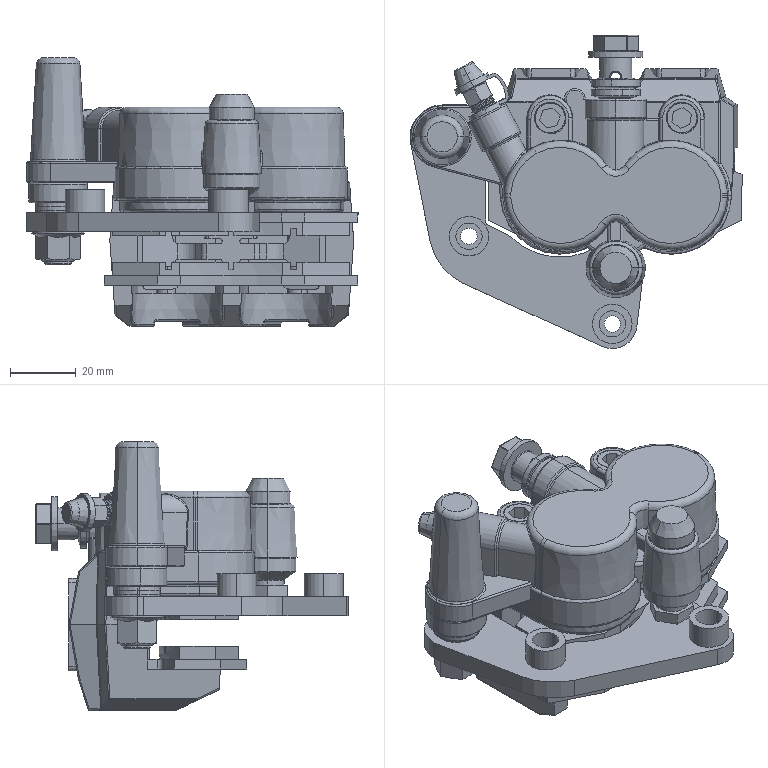Part | SolidWorks | 20 solids | 1156 faces | box 100.773 x 95.04 x 81.512 mm | volume 159092 mm3 | cylinder 505 | plane 380 | torus 88 | cone 78 | spline 70 | sphere 35 | commonest cylinder face diameters 1 x112 8 x38 9.8 x38 4 x27 9.82 x24 2 x19